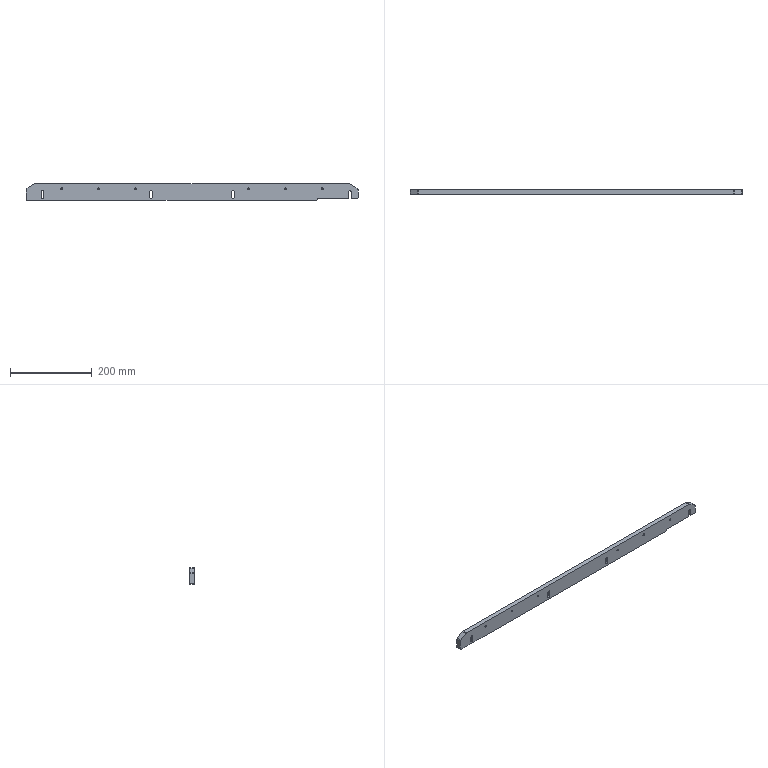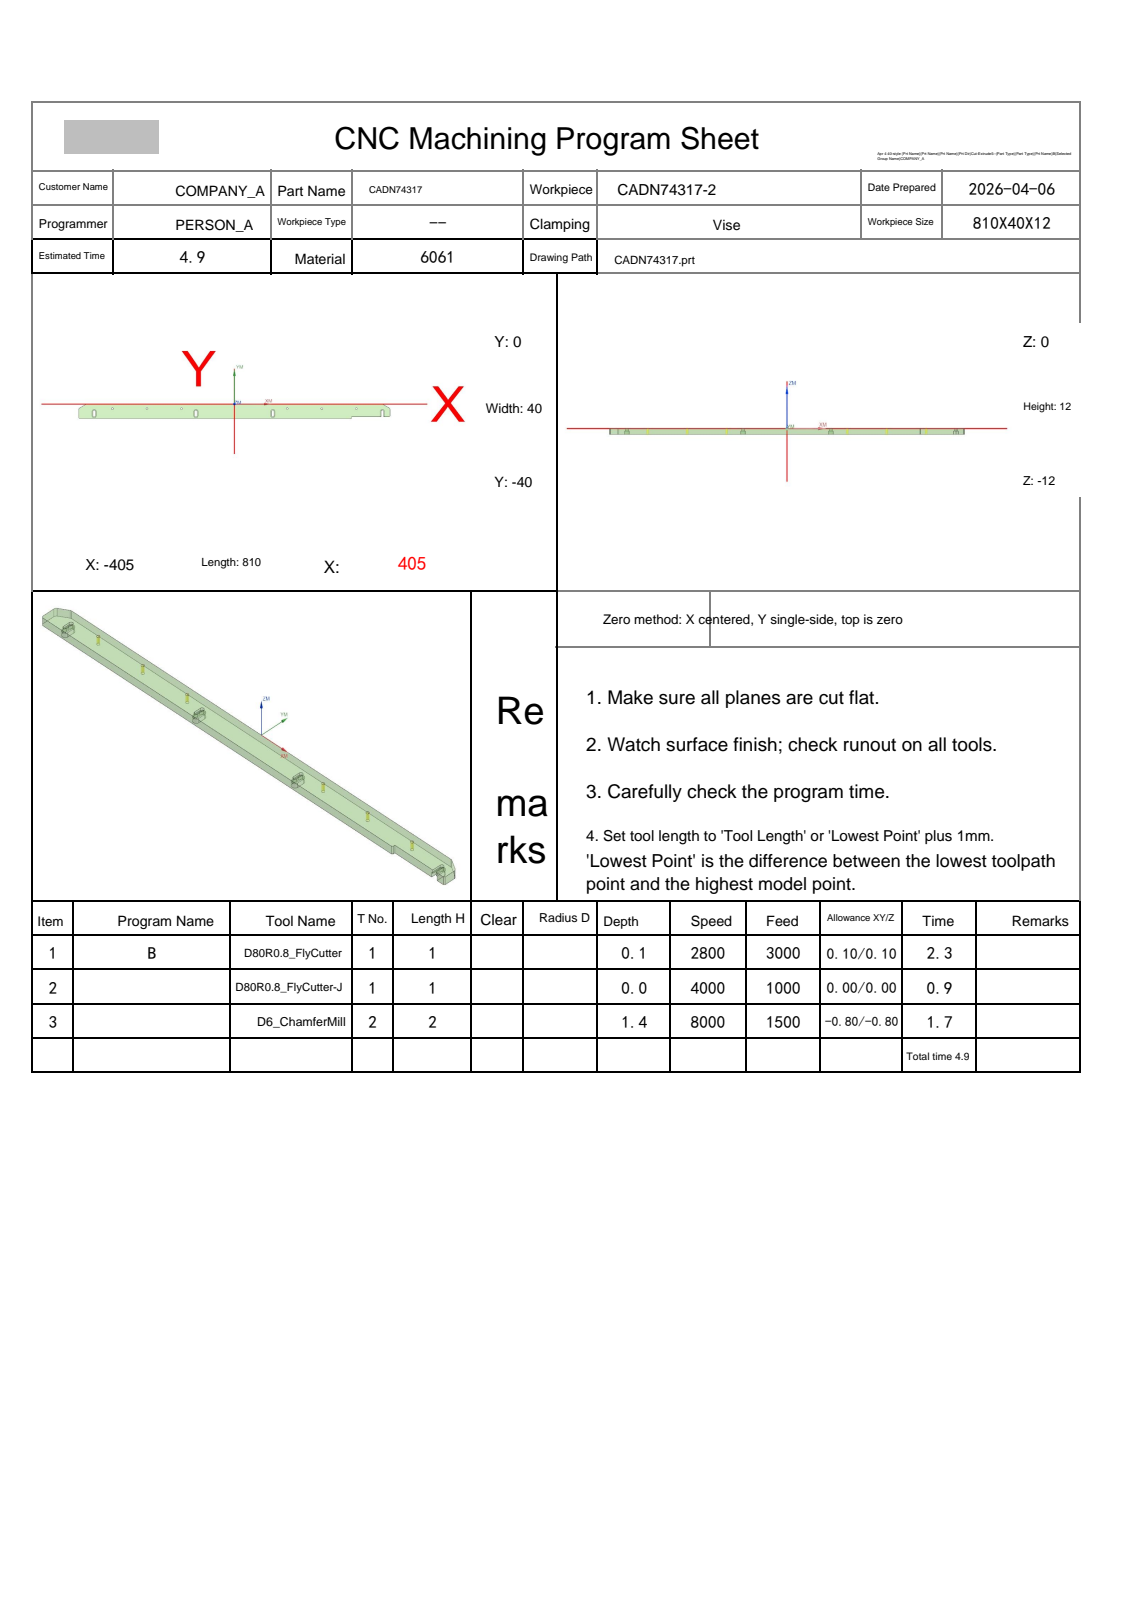NC program | NX | posted by the shop | part box 810 x 12 x 40 mm
Whole program:
%
O0001
(Machine time: 5.41 MIN)
(===Total Tool:2===)
(T1=D80R0.8 FlyCutter D=80.  R=0.8  D-  H01 Z=0.    )
(T2=D6_ChamferMill   D=6.   R=0.   D-  H02 Z=-1.4  )
G80 G90 G17 G49 G40
G91 G28 Z0
M01
N1 T01 M06
(D80R0.8 FlyCutter  D=80. R=0.8 H=01 ce=0.10 di=0.10)
G00 G90 G54 X457.086 Y-13.704 M03 S2800
G43 H01 Z20.
M08
Z4.35
G01 Z2.35 F3000.
X445.086 Y-13.856
X-445.097 Y-25.124
X-457.097 Y-25.275
Z4.35
G00 X457.086 Y-13.704
Z3.9
G01 Z1.9
X445.086 Y-13.856
X-445.097 Y-25.124
X-457.097 Y-25.275
Z3.9
G00 X457.086 Y-13.704
Z3.45
G01 Z1.45
X445.086 Y-13.856
X-445.097 Y-25.124
X-457.097 Y-25.275
Z3.45
G00 X457.086 Y-13.704
Z3.
G01 Z1.
X445.086 Y-13.856
X-445.097 Y-25.124
X-457.097 Y-25.275
Z3.
G00 Z20.
X457.086 Y-13.704
Z2.55
G01 Z.55
X445.086 Y-13.856
X-445.097 Y-25.124
X-457.097 Y-25.275
Z2.55
G00 Z20.
X457.086 Y-13.704
Z2.1
G01 Z.1
X445.086 Y-13.856
X-445.097 Y-25.124
X-457.097 Y-25.275
Z2.1
G00 Z20.
G91 G28 Z0.0
M05
M09
G91 G28 Z0.0
M01
N2 T01 M06
(D80R0.8 FlyCutter-J  D=80. R=0.8 H=01 ce=0.00 di=0.00)
G00 G90 G54 X456.988 Y-13.72 M03 S4000
G43 H01 Z20.
M08
Z2.
G01 Z0.0 F1000.
X444.989 Y-13.872
X-444.999 Y-25.11
X-456.999 Y-25.262
Z2.
G00 Z20.
G91 G28 Z0.0
M05
M09
G91 G28 Z0.0
M01
N3 T02 M06
(D6_ChamferMill  D=6. R=0. H=02 ce=-0.80 di=-0.80)
G00 G90 G54 X-316.63 Y-12.268 M03 S8000
G43 H02 Z20.
M08
Z-.9
G01 Z-1.4 F600.
X-316. Y-12.1
G03 X-317.5 Y-10.6 I-1.5 J0.0
X-319.4 Y-12.5 I0.0 J-1.9
X-317.5 Y-14.4 I1.9 J0.0
X-315.6 Y-12.5 I0.0 J1.9
X-317.5 Y-10.6 I-1.9 J0.0
X-319. Y-12.1 I0.0 J-1.5
G01 X-318.37 Y-12.268
Z-.9
G00 Z20.
X-226.63
Z-.9
G01 Z-1.4
X-226. Y-12.1
G03 X-227.5 Y-10.6 I-1.5 J0.0
X-229.4 Y-12.5 I0.0 J-1.9
X-227.5 Y-14.4 I1.9 J0.0
X-225.6 Y-12.5 I0.0 J1.9
X-227.5 Y-10.6 I-1.9 J0.0
X-229. Y-12.1 I0.0 J-1.5
G01 X-228.37 Y-12.268
Z-.9
G00 Z20.
X-136.63
Z-.9
G01 Z-1.4
X-136. Y-12.1
G03 X-137.5 Y-10.6 I-1.5 J0.0
X-139.4 Y-12.5 I0.0 J-1.9
X-137.5 Y-14.4 I1.9 J0.0
X-135.6 Y-12.5 I0.0 J1.9
X-137.5 Y-10.6 I-1.9 J0.0
X-139. Y-12.1 I0.0 J-1.5
G01 X-138.37 Y-12.268
Z-.9
G00 Z20.
X138.37
Z-.9
G01 Z-1.4
X139. Y-12.1
G03 X137.5 Y-10.6 I-1.5 J0.0
X135.6 Y-12.5 I0.0 J-1.9
X137.5 Y-14.4 I1.9 J0.0
X139.4 Y-12.5 I0.0 J1.9
X137.5 Y-10.6 I-1.9 J0.0
X136. Y-12.1 I0.0 J-1.5
G01 X136.63 Y-12.268
Z-.9
G00 Z20.
X228.37
Z-.9
G01 Z-1.4
X229. Y-12.1
G03 X227.5 Y-10.6 I-1.5 J0.0
X225.6 Y-12.5 I0.0 J-1.9
X227.5 Y-14.4 I1.9 J0.0
X229.4 Y-12.5 I0.0 J1.9
X227.5 Y-10.6 I-1.9 J0.0
X226. Y-12.1 I0.0 J-1.5
G01 X226.63 Y-12.268
Z-.9
G00 Z20.
X318.37
Z-.9
G01 Z-1.4
X319. Y-12.1
G03 X317.5 Y-10.6 I-1.5 J0.0
X315.6 Y-12.5 I0.0 J-1.9
X317.5 Y-14.4 I1.9 J0.0
X319.4 Y-12.5 I0.0 J1.9
X317.5 Y-10.6 I-1.9 J0.0
X316. Y-12.1 I0.0 J-1.5
G01 X316.63 Y-12.268
Z-.9
G00 Z20.
G00 G90 X-.386 Y1.227 M03 S6500
Z20.
Z.172
G01 Z-1.2 F1500.
G03 X-.1 Y1.027 I1.286 J1.532
G01 X-.054 Y.997
X0.0 Y1.
X383.615
G02 X386.702 Y.145 I0.0 J-6.
G01 X403.087 Y-9.686
G02 X406. Y-14.831 I-3.087 J-5.145
G01 Y-33.
X405.966 Y-33.259
X405.866 Y-33.5
X405.707 Y-33.707
X403.707 Y-35.707
X403.5 Y-35.866
X403.259 Y-35.966
X403. Y-36.
X388.3
G02 X387.3 Y-35. I0.0 J1.
G01 Y-20.
G03 X385. Y-17.7 I-2.3 J0.0
X382.7 Y-20. I0.0 J-2.3
G01 Y-35.
G02 X381.7 Y-36. I-1. J0.0
G01 X306.
Y-38.
X305.966 Y-38.259
X305.866 Y-38.5
X305.707 Y-38.707
X303.707 Y-40.707
X303.5 Y-40.866
X303.259 Y-40.966
X303. Y-41.
X-403.
X-403.259 Y-40.966
X-403.5 Y-40.866
X-403.707 Y-40.707
X-405.707 Y-38.707
X-405.866 Y-38.5
X-405.966 Y-38.259
X-406. Y-38.
Y-14.831
G02 X-403.087 Y-9.686 I6. J0.0
G01 X-386.702 Y.145
G02 X-383.615 Y1. I3.087 J-5.145
G01 X0.0
X.054 Y.997
X.1 Y1.027
G03 X.386 Y1.227 I-1. J1.732
G01 Z.172
G00 Z10.
X317.907 Y-11.185
Z.284
G01 Z-1.2
G03 X317.602 Y-11.016 I-1.118 J-1.658
G01 X317.554 Y-10.991
X317.5 Y-11.
G03 X316. Y-12.5 I0.0 J-1.5
X317.5 Y-14. I1.5 J0.0
X319. Y-12.5 I0.0 J1.5
X317.5 Y-11. I-1.5 J0.0
G01 X317.446 Y-10.991
X317.398 Y-11.016
G03 X317.093 Y-11.185 I.813 J-1.827
G01 Z.284
G00 Z10.
X227.907
Z.284
G01 Z-1.2
G03 X227.602 Y-11.016 I-1.118 J-1.658
G01 X227.554 Y-10.991
X227.5 Y-11.
G03 X226. Y-12.5 I0.0 J-1.5
X227.5 Y-14. I1.5 J0.0
X229. Y-12.5 I0.0 J1.5
X227.5 Y-11. I-1.5 J0.0
G01 X227.446 Y-10.991
X227.398 Y-11.016
G03 X227.093 Y-11.185 I.813 J-1.827
G01 Z.284
G00 Z10.
X137.907
Z.284
G01 Z-1.2
G03 X137.602 Y-11.016 I-1.118 J-1.658
G01 X137.554 Y-10.991
X137.5 Y-11.
G03 X136. Y-12.5 I0.0 J-1.5
X137.5 Y-14. I1.5 J0.0
X139. Y-12.5 I0.0 J1.5
X137.5 Y-11. I-1.5 J0.0
G01 X137.446 Y-10.991
X137.398 Y-11.016
G03 X137.093 Y-11.185 I.813 J-1.827
G01 Z.284
G00 Z10.
X97.927 Y-25.614
Z.172
G01 Z-1.2
G03 X97.727 Y-25.9 I1.532 J-1.286
G01 X97.697 Y-25.946
X97.7 Y-26.
Y-32.
G03 X100. Y-34.3 I2.3 J0.0
X102.3 Y-32. I0.0 J2.3
G01 Y-20.
G03 X100. Y-17.7 I-2.3 J0.0
X97.7 Y-20. I0.0 J-2.3
G01 Y-26.
X97.697 Y-26.054
X97.727 Y-26.1
G03 X97.927 Y-26.386 I1.732 J1.
G01 Z.172
G00 Z10.
X-97.927
Z.172
G01 Z-1.2
G03 X-97.727 Y-26.1 I-1.532 J1.286
G01 X-97.697 Y-26.054
X-97.7 Y-26.
Y-20.
G03 X-100. Y-17.7 I-2.3 J0.0
X-102.3 Y-20. I0.0 J-2.3
G01 Y-32.
G03 X-100. Y-34.3 I2.3 J0.0
X-97.7 Y-32. I0.0 J2.3
G01 Y-26.
X-97.697 Y-25.946
X-97.727 Y-25.9
G03 X-97.927 Y-25.614 I-1.732 J-1.
G01 Z.172
G00 Z10.
X-137.093 Y-11.185
Z.284
G01 Z-1.2
G03 X-137.398 Y-11.016 I-1.118 J-1.658
G01 X-137.446 Y-10.991
X-137.5 Y-11.
G03 X-139. Y-12.5 I0.0 J-1.5
X-137.5 Y-14. I1.5 J0.0
X-136. Y-12.5 I0.0 J1.5
X-137.5 Y-11. I-1.5 J0.0
G01 X-137.554 Y-10.991
X-137.602 Y-11.016
G03 X-137.907 Y-11.185 I.813 J-1.827
G01 Z.284
G00 Z10.
X-227.093
Z.284
G01 Z-1.2
G03 X-227.398 Y-11.016 I-1.118 J-1.658
G01 X-227.446 Y-10.991
X-227.5 Y-11.
G03 X-229. Y-12.5 I0.0 J-1.5
X-227.5 Y-14. I1.5 J0.0
X-226. Y-12.5 I0.0 J1.5
X-227.5 Y-11. I-1.5 J0.0
G01 X-227.554 Y-10.991
X-227.602 Y-11.016
G03 X-227.907 Y-11.185 I.813 J-1.827
G01 Z.284
G00 Z10.
X-317.093
Z.284
G01 Z-1.2
G03 X-317.398 Y-11.016 I-1.118 J-1.658
G01 X-317.446 Y-10.991
X-317.5 Y-11.
G03 X-319. Y-12.5 I0.0 J-1.5
X-317.5 Y-14. I1.5 J0.0
X-316. Y-12.5 I0.0 J1.5
X-317.5 Y-11. I-1.5 J0.0
G01 X-317.554 Y-10.991
X-317.602 Y-11.016
G03 X-317.907 Y-11.185 I.813 J-1.827
G01 Z.284
G00 Z10.
X-362.927 Y-26.386
Z.172
G01 Z-1.2
G03 X-362.727 Y-26.1 I-1.532 J1.286
G01 X-362.697 Y-26.054
X-362.7 Y-26.
Y-20.
G03 X-365. Y-17.7 I-2.3 J0.0
X-367.3 Y-20. I0.0 J-2.3
G01 Y-32.
G03 X-365. Y-34.3 I2.3 J0.0
X-362.7 Y-32. I0.0 J2.3
G01 Y-26.
X-362.697 Y-25.946
X-362.727 Y-25.9
G03 X-362.927 Y-25.614 I-1.732 J-1.
G01 Z.172
G00 Z20.
M05
M09
G91 G28 Z0.0
G91 G28 Y0.0
M30
%